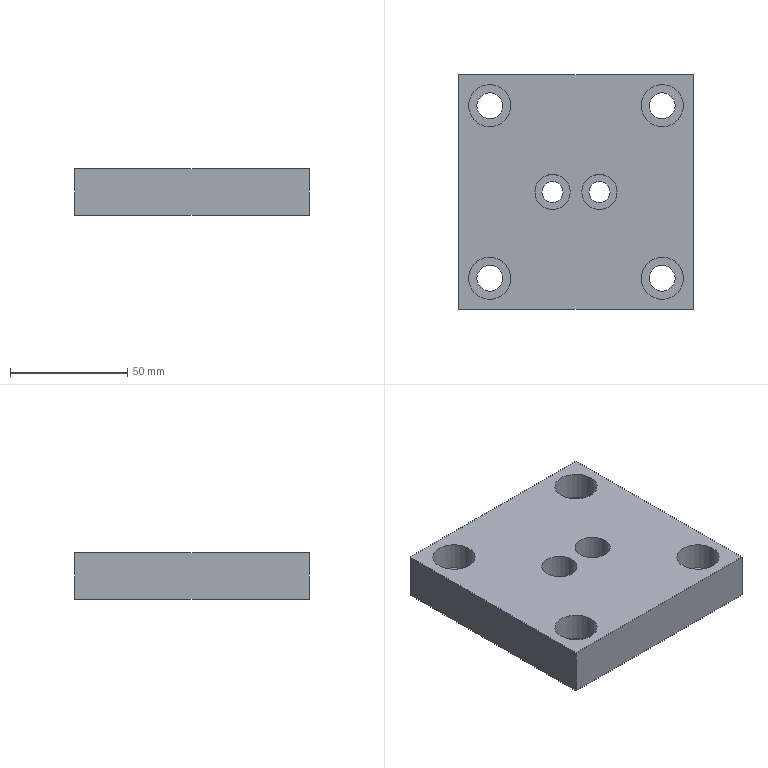Part | NX | features 1 2 | 1 solid | 24 faces | box 100 x 100 x 19.8 mm | volume 177134 mm3 | cylinder 12 | plane 12 | commonest cylinder face diameters 11 x4 18 x4 9 x2 15 x2
STEP:
#1=CARTESIAN_POINT('',(797.75,188.25,343.));
#2=VERTEX_POINT('',#1);
#3=CARTESIAN_POINT('',(806.75,188.25,343.));
#4=DIRECTION('',(0.,0.,-1.));
#5=DIRECTION('',(-1.,0.,0.));
#6=AXIS2_PLACEMENT_3D('',#3,#4,#5);
#7=CIRCLE('',#6,9.);
#8=EDGE_CURVE('',#2,#2,#7,.T.);
#9=ORIENTED_EDGE('',*,*,#8,.T.);
#10=EDGE_LOOP('',(#9));
#11=FACE_BOUND('',#10,.T.);
#12=CARTESIAN_POINT('',(797.75,188.25,355.));
#13=VERTEX_POINT('',#12);
#14=CARTESIAN_POINT('',(806.75,188.25,355.));
#15=DIRECTION('',(0.,0.,1.));
#16=DIRECTION('',(-1.,0.,0.));
#17=AXIS2_PLACEMENT_3D('',#14,#15,#16);
#18=CIRCLE('',#17,9.);
#19=EDGE_CURVE('',#13,#13,#18,.T.);
#20=ORIENTED_EDGE('',*,*,#19,.T.);
#21=EDGE_LOOP('',(#20));
#22=FACE_BOUND('',#21,.T.);
#23=CARTESIAN_POINT('',(806.75,188.25,355.));
#24=DIRECTION('',(0.,0.,1.));
#25=DIRECTION('',(0.,-1.,0.));
#26=AXIS2_PLACEMENT_3D('',#23,#24,#25);
#27=CYLINDRICAL_SURFACE('',#26,9.);
#28=ADVANCED_FACE('',(#11,#22),#27,.F.);
#29=CARTESIAN_POINT('',(801.25,188.25,335.2));
#30=VERTEX_POINT('',#29);
#31=CARTESIAN_POINT('',(806.75,188.25,335.2));
#32=DIRECTION('',(0.,0.,-1.));
#33=DIRECTION('',(-1.,0.,0.));
#34=AXIS2_PLACEMENT_3D('',#31,#32,#33);
#35=CIRCLE('',#34,5.5);
#36=EDGE_CURVE('',#30,#30,#35,.T.);
#37=ORIENTED_EDGE('',*,*,#36,.T.);
#38=EDGE_LOOP('',(#37));
#39=FACE_BOUND('',#38,.T.);
#40=CARTESIAN_POINT('',(801.25,188.25,343.));
#41=VERTEX_POINT('',#40);
#42=CARTESIAN_POINT('',(806.75,188.25,343.));
#43=DIRECTION('',(0.,0.,1.));
#44=DIRECTION('',(-1.,0.,0.));
#45=AXIS2_PLACEMENT_3D('',#42,#43,#44);
#46=CIRCLE('',#45,5.5);
#47=EDGE_CURVE('',#41,#41,#46,.T.);
#48=ORIENTED_EDGE('',*,*,#47,.T.);
#49=EDGE_LOOP('',(#48));
#50=FACE_BOUND('',#49,.T.);
#51=CARTESIAN_POINT('',(806.75,188.25,343.));
#52=DIRECTION('',(0.,0.,1.));
#53=DIRECTION('',(0.,-1.,0.));
#54=AXIS2_PLACEMENT_3D('',#51,#52,#53);
#55=CYLINDRICAL_SURFACE('',#54,5.5);
#56=ADVANCED_FACE('',(#39,#50),#55,.F.);
#57=CARTESIAN_POINT('',(724.25,188.25,343.));
#58=VERTEX_POINT('',#57);
#59=CARTESIAN_POINT('',(733.25,188.25,343.));
#60=DIRECTION('',(0.,0.,-1.));
#61=DIRECTION('',(-1.,0.,0.));
#62=AXIS2_PLACEMENT_3D('',#59,#60,#61);
#63=CIRCLE('',#62,9.);
#64=EDGE_CURVE('',#58,#58,#63,.T.);
#65=ORIENTED_EDGE('',*,*,#64,.T.);
#66=EDGE_LOOP('',(#65));
#67=FACE_BOUND('',#66,.T.);
#68=CARTESIAN_POINT('',(724.25,188.25,355.));
#69=VERTEX_POINT('',#68);
#70=CARTESIAN_POINT('',(733.25,188.25,355.));
#71=DIRECTION('',(0.,0.,1.));
#72=DIRECTION('',(-1.,0.,0.));
#73=AXIS2_PLACEMENT_3D('',#70,#71,#72);
#74=CIRCLE('',#73,9.);
#75=EDGE_CURVE('',#69,#69,#74,.T.);
#76=ORIENTED_EDGE('',*,*,#75,.T.);
#77=EDGE_LOOP('',(#76));
#78=FACE_BOUND('',#77,.T.);
#79=CARTESIAN_POINT('',(733.25,188.25,355.));
#80=DIRECTION('',(0.,0.,1.));
#81=DIRECTION('',(0.,-1.,0.));
#82=AXIS2_PLACEMENT_3D('',#79,#80,#81);
#83=CYLINDRICAL_SURFACE('',#82,9.);
#84=ADVANCED_FACE('',(#67,#78),#83,.F.);
#85=CARTESIAN_POINT('',(727.75,188.25,335.2));
#86=VERTEX_POINT('',#85);
#87=CARTESIAN_POINT('',(733.25,188.25,335.2));
#88=DIRECTION('',(0.,0.,-1.));
#89=DIRECTION('',(-1.,0.,0.));
#90=AXIS2_PLACEMENT_3D('',#87,#88,#89);
#91=CIRCLE('',#90,5.5);
#92=EDGE_CURVE('',#86,#86,#91,.T.);
#93=ORIENTED_EDGE('',*,*,#92,.T.);
#94=EDGE_LOOP('',(#93));
#95=FACE_BOUND('',#94,.T.);
#96=CARTESIAN_POINT('',(727.75,188.25,343.));
#97=VERTEX_POINT('',#96);
#98=CARTESIAN_POINT('',(733.25,188.25,343.));
#99=DIRECTION('',(0.,0.,1.));
#100=DIRECTION('',(-1.,0.,0.));
#101=AXIS2_PLACEMENT_3D('',#98,#99,#100);
#102=CIRCLE('',#101,5.5);
#103=EDGE_CURVE('',#97,#97,#102,.T.);
#104=ORIENTED_EDGE('',*,*,#103,.T.);
#105=EDGE_LOOP('',(#104));
#106=FACE_BOUND('',#105,.T.);
#107=CARTESIAN_POINT('',(733.25,188.25,343.));
#108=DIRECTION('',(0.,0.,1.));
#109=DIRECTION('',(0.,-1.,0.));
#110=AXIS2_PLACEMENT_3D('',#107,#108,#109);
#111=CYLINDRICAL_SURFACE('',#110,5.5);
#112=ADVANCED_FACE('',(#95,#106),#111,.F.);
#113=CARTESIAN_POINT('',(797.75,261.75,343.));
#114=VERTEX_POINT('',#113);
#115=CARTESIAN_POINT('',(806.75,261.75,343.));
#116=DIRECTION('',(0.,0.,-1.));
#117=DIRECTION('',(-1.,0.,0.));
#118=AXIS2_PLACEMENT_3D('',#115,#116,#117);
#119=CIRCLE('',#118,9.);
#120=EDGE_CURVE('',#114,#114,#119,.T.);
#121=ORIENTED_EDGE('',*,*,#120,.T.);
#122=EDGE_LOOP('',(#121));
#123=FACE_BOUND('',#122,.T.);
#124=CARTESIAN_POINT('',(797.75,261.75,355.));
#125=VERTEX_POINT('',#124);
#126=CARTESIAN_POINT('',(806.75,261.75,355.));
#127=DIRECTION('',(0.,0.,1.));
#128=DIRECTION('',(-1.,0.,0.));
#129=AXIS2_PLACEMENT_3D('',#126,#127,#128);
#130=CIRCLE('',#129,9.);
#131=EDGE_CURVE('',#125,#125,#130,.T.);
#132=ORIENTED_EDGE('',*,*,#131,.T.);
#133=EDGE_LOOP('',(#132));
#134=FACE_BOUND('',#133,.T.);
#135=CARTESIAN_POINT('',(806.75,261.75,355.));
#136=DIRECTION('',(0.,0.,1.));
#137=DIRECTION('',(0.,-1.,0.));
#138=AXIS2_PLACEMENT_3D('',#135,#136,#137);
#139=CYLINDRICAL_SURFACE('',#138,9.);
#140=ADVANCED_FACE('',(#123,#134),#139,.F.);
#141=CARTESIAN_POINT('',(801.25,261.75,335.2));
#142=VERTEX_POINT('',#141);
#143=CARTESIAN_POINT('',(806.75,261.75,335.2));
#144=DIRECTION('',(0.,0.,-1.));
#145=DIRECTION('',(-1.,0.,0.));
#146=AXIS2_PLACEMENT_3D('',#143,#144,#145);
#147=CIRCLE('',#146,5.5);
#148=EDGE_CURVE('',#142,#142,#147,.T.);
#149=ORIENTED_EDGE('',*,*,#148,.T.);
#150=EDGE_LOOP('',(#149));
#151=FACE_BOUND('',#150,.T.);
#152=CARTESIAN_POINT('',(801.25,261.75,343.));
#153=VERTEX_POINT('',#152);
#154=CARTESIAN_POINT('',(806.75,261.75,343.));
#155=DIRECTION('',(0.,0.,1.));
#156=DIRECTION('',(-1.,0.,0.));
#157=AXIS2_PLACEMENT_3D('',#154,#155,#156);
#158=CIRCLE('',#157,5.5);
#159=EDGE_CURVE('',#153,#153,#158,.T.);
#160=ORIENTED_EDGE('',*,*,#159,.T.);
#161=EDGE_LOOP('',(#160));
#162=FACE_BOUND('',#161,.T.);
#163=CARTESIAN_POINT('',(806.75,261.75,343.));
#164=DIRECTION('',(0.,0.,1.));
#165=DIRECTION('',(0.,-1.,0.));
#166=AXIS2_PLACEMENT_3D('',#163,#164,#165);
#167=CYLINDRICAL_SURFACE('',#166,5.5);
#168=ADVANCED_FACE('',(#151,#162),#167,.F.);
#169=CARTESIAN_POINT('',(724.25,261.75,343.));
#170=VERTEX_POINT('',#169);
#171=CARTESIAN_POINT('',(733.25,261.75,343.));
#172=DIRECTION('',(0.,0.,-1.));
#173=DIRECTION('',(-1.,0.,0.));
#174=AXIS2_PLACEMENT_3D('',#171,#172,#173);
#175=CIRCLE('',#174,9.);
#176=EDGE_CURVE('',#170,#170,#175,.T.);
#177=ORIENTED_EDGE('',*,*,#176,.T.);
#178=EDGE_LOOP('',(#177));
#179=FACE_BOUND('',#178,.T.);
#180=CARTESIAN_POINT('',(724.25,261.75,355.));
#181=VERTEX_POINT('',#180);
#182=CARTESIAN_POINT('',(733.25,261.75,355.));
#183=DIRECTION('',(0.,0.,1.));
#184=DIRECTION('',(-1.,0.,0.));
#185=AXIS2_PLACEMENT_3D('',#182,#183,#184);
#186=CIRCLE('',#185,9.);
#187=EDGE_CURVE('',#181,#181,#186,.T.);
#188=ORIENTED_EDGE('',*,*,#187,.T.);
#189=EDGE_LOOP('',(#188));
#190=FACE_BOUND('',#189,.T.);
#191=CARTESIAN_POINT('',(733.25,261.75,355.));
#192=DIRECTION('',(0.,0.,1.));
#193=DIRECTION('',(0.,-1.,0.));
#194=AXIS2_PLACEMENT_3D('',#191,#192,#193);
#195=CYLINDRICAL_SURFACE('',#194,9.);
#196=ADVANCED_FACE('',(#179,#190),#195,.F.);
#197=CARTESIAN_POINT('',(727.75,261.75,335.2));
#198=VERTEX_POINT('',#197);
#199=CARTESIAN_POINT('',(733.25,261.75,335.2));
#200=DIRECTION('',(0.,0.,-1.));
#201=DIRECTION('',(-1.,0.,0.));
#202=AXIS2_PLACEMENT_3D('',#199,#200,#201);
#203=CIRCLE('',#202,5.5);
#204=EDGE_CURVE('',#198,#198,#203,.T.);
#205=ORIENTED_EDGE('',*,*,#204,.T.);
#206=EDGE_LOOP('',(#205));
#207=FACE_BOUND('',#206,.T.);
#208=CARTESIAN_POINT('',(727.75,261.75,343.));
#209=VERTEX_POINT('',#208);
#210=CARTESIAN_POINT('',(733.25,261.75,343.));
#211=DIRECTION('',(0.,0.,1.));
#212=DIRECTION('',(-1.,0.,0.));
#213=AXIS2_PLACEMENT_3D('',#210,#211,#212);
#214=CIRCLE('',#213,5.5);
#215=EDGE_CURVE('',#209,#209,#214,.T.);
#216=ORIENTED_EDGE('',*,*,#215,.T.);
#217=EDGE_LOOP('',(#216));
#218=FACE_BOUND('',#217,.T.);
#219=CARTESIAN_POINT('',(733.25,261.75,343.));
#220=DIRECTION('',(0.,0.,1.));
#221=DIRECTION('',(0.,-1.,0.));
#222=AXIS2_PLACEMENT_3D('',#219,#220,#221);
#223=CYLINDRICAL_SURFACE('',#222,5.5);
#224=ADVANCED_FACE('',(#207,#218),#223,.F.);
#225=CARTESIAN_POINT('',(772.5,225.,341.));
#226=VERTEX_POINT('',#225);
#227=CARTESIAN_POINT('',(780.,225.,341.));
#228=DIRECTION('',(0.,0.,-1.));
#229=DIRECTION('',(-1.,0.,0.));
#230=AXIS2_PLACEMENT_3D('',#227,#228,#229);
#231=CIRCLE('',#230,7.5);
#232=EDGE_CURVE('',#226,#226,#231,.T.);
#233=ORIENTED_EDGE('',*,*,#232,.T.);
#234=EDGE_LOOP('',(#233));
#235=FACE_BOUND('',#234,.T.);
#236=CARTESIAN_POINT('',(772.5,225.,355.));
#237=VERTEX_POINT('',#236);
#238=CARTESIAN_POINT('',(780.,225.,355.));
#239=DIRECTION('',(0.,0.,1.));
#240=DIRECTION('',(-1.,0.,0.));
#241=AXIS2_PLACEMENT_3D('',#238,#239,#240);
#242=CIRCLE('',#241,7.5);
#243=EDGE_CURVE('',#237,#237,#242,.T.);
#244=ORIENTED_EDGE('',*,*,#243,.T.);
#245=EDGE_LOOP('',(#244));
#246=FACE_BOUND('',#245,.T.);
#247=CARTESIAN_POINT('',(780.,225.,355.));
#248=DIRECTION('',(0.,0.,1.));
#249=DIRECTION('',(0.,-1.,0.));
#250=AXIS2_PLACEMENT_3D('',#247,#248,#249);
#251=CYLINDRICAL_SURFACE('',#250,7.5);
#252=ADVANCED_FACE('',(#235,#246),#251,.F.);
#253=CARTESIAN_POINT('',(775.5,225.,335.2));
#254=VERTEX_POINT('',#253);
#255=CARTESIAN_POINT('',(780.,225.,335.2));
#256=DIRECTION('',(0.,0.,-1.));
#257=DIRECTION('',(-1.,0.,0.));
#258=AXIS2_PLACEMENT_3D('',#255,#256,#257);
#259=CIRCLE('',#258,4.5);
#260=EDGE_CURVE('',#254,#254,#259,.T.);
#261=ORIENTED_EDGE('',*,*,#260,.T.);
#262=EDGE_LOOP('',(#261));
#263=FACE_BOUND('',#262,.T.);
#264=CARTESIAN_POINT('',(775.5,225.,341.));
#265=VERTEX_POINT('',#264);
#266=CARTESIAN_POINT('',(780.,225.,341.));
#267=DIRECTION('',(0.,0.,1.));
#268=DIRECTION('',(-1.,0.,0.));
#269=AXIS2_PLACEMENT_3D('',#266,#267,#268);
#270=CIRCLE('',#269,4.5);
#271=EDGE_CURVE('',#265,#265,#270,.T.);
#272=ORIENTED_EDGE('',*,*,#271,.T.);
#273=EDGE_LOOP('',(#272));
#274=FACE_BOUND('',#273,.T.);
#275=CARTESIAN_POINT('',(780.,225.,341.));
#276=DIRECTION('',(0.,0.,1.));
#277=DIRECTION('',(0.,-1.,0.));
#278=AXIS2_PLACEMENT_3D('',#275,#276,#277);
#279=CYLINDRICAL_SURFACE('',#278,4.5);
#280=ADVANCED_FACE('',(#263,#274),#279,.F.);
#281=CARTESIAN_POINT('',(752.5,225.,341.));
#282=VERTEX_POINT('',#281);
#283=CARTESIAN_POINT('',(760.,225.,341.));
#284=DIRECTION('',(0.,0.,-1.));
#285=DIRECTION('',(-1.,0.,0.));
#286=AXIS2_PLACEMENT_3D('',#283,#284,#285);
#287=CIRCLE('',#286,7.5);
#288=EDGE_CURVE('',#282,#282,#287,.T.);
#289=ORIENTED_EDGE('',*,*,#288,.T.);
#290=EDGE_LOOP('',(#289));
#291=FACE_BOUND('',#290,.T.);
#292=CARTESIAN_POINT('',(752.5,225.,355.));
#293=VERTEX_POINT('',#292);
#294=CARTESIAN_POINT('',(760.,225.,355.));
#295=DIRECTION('',(0.,0.,1.));
#296=DIRECTION('',(-1.,0.,0.));
#297=AXIS2_PLACEMENT_3D('',#294,#295,#296);
#298=CIRCLE('',#297,7.5);
#299=EDGE_CURVE('',#293,#293,#298,.T.);
#300=ORIENTED_EDGE('',*,*,#299,.T.);
#301=EDGE_LOOP('',(#300));
#302=FACE_BOUND('',#301,.T.);
#303=CARTESIAN_POINT('',(760.,225.,355.));
#304=DIRECTION('',(0.,0.,1.));
#305=DIRECTION('',(0.,-1.,0.));
#306=AXIS2_PLACEMENT_3D('',#303,#304,#305);
#307=CYLINDRICAL_SURFACE('',#306,7.5);
#308=ADVANCED_FACE('',(#291,#302),#307,.F.);
#309=CARTESIAN_POINT('',(755.5,225.,335.2));
#310=VERTEX_POINT('',#309);
#311=CARTESIAN_POINT('',(760.,225.,335.2));
#312=DIRECTION('',(0.,0.,-1.));
#313=DIRECTION('',(-1.,0.,0.));
#314=AXIS2_PLACEMENT_3D('',#311,#312,#313);
#315=CIRCLE('',#314,4.5);
#316=EDGE_CURVE('',#310,#310,#315,.T.);
#317=ORIENTED_EDGE('',*,*,#316,.T.);
#318=EDGE_LOOP('',(#317));
#319=FACE_BOUND('',#318,.T.);
#320=CARTESIAN_POINT('',(755.5,225.,341.));
#321=VERTEX_POINT('',#320);
#322=CARTESIAN_POINT('',(760.,225.,341.));
#323=DIRECTION('',(0.,0.,1.));
#324=DIRECTION('',(-1.,0.,0.));
#325=AXIS2_PLACEMENT_3D('',#322,#323,#324);
#326=CIRCLE('',#325,4.5);
#327=EDGE_CURVE('',#321,#321,#326,.T.);
#328=ORIENTED_EDGE('',*,*,#327,.T.);
#329=EDGE_LOOP('',(#328));
#330=FACE_BOUND('',#329,.T.);
#331=CARTESIAN_POINT('',(760.,225.,341.));
#332=DIRECTION('',(0.,0.,1.));
#333=DIRECTION('',(0.,-1.,0.));
#334=AXIS2_PLACEMENT_3D('',#331,#332,#333);
#335=CYLINDRICAL_SURFACE('',#334,4.5);
#336=ADVANCED_FACE('',(#319,#330),#335,.F.);
#337=ORIENTED_EDGE('',*,*,#327,.F.);
#338=EDGE_LOOP('',(#337));
#339=FACE_BOUND('',#338,.T.);
#340=ORIENTED_EDGE('',*,*,#288,.F.);
#341=EDGE_LOOP('',(#340));
#342=FACE_BOUND('',#341,.T.);
#343=CARTESIAN_POINT('',(820.,175.,341.));
#344=DIRECTION('',(0.,0.,1.));
#345=DIRECTION('',(0.,-1.,0.));
#346=AXIS2_PLACEMENT_3D('',#343,#344,#345);
#347=PLANE('',#346);
#348=ADVANCED_FACE('',(#339,#342),#347,.T.);
#349=ORIENTED_EDGE('',*,*,#271,.F.);
#350=EDGE_LOOP('',(#349));
#351=FACE_BOUND('',#350,.T.);
#352=ORIENTED_EDGE('',*,*,#232,.F.);
#353=EDGE_LOOP('',(#352));
#354=FACE_BOUND('',#353,.T.);
#355=CARTESIAN_POINT('',(820.,175.,341.));
#356=DIRECTION('',(0.,0.,1.));
#357=DIRECTION('',(0.,-1.,0.));
#358=AXIS2_PLACEMENT_3D('',#355,#356,#357);
#359=PLANE('',#358);
#360=ADVANCED_FACE('',(#351,#354),#359,.T.);
#361=ORIENTED_EDGE('',*,*,#215,.F.);
#362=EDGE_LOOP('',(#361));
#363=FACE_BOUND('',#362,.T.);
#364=ORIENTED_EDGE('',*,*,#176,.F.);
#365=EDGE_LOOP('',(#364));
#366=FACE_BOUND('',#365,.T.);
#367=CARTESIAN_POINT('',(820.,175.,343.));
#368=DIRECTION('',(0.,0.,1.));
#369=DIRECTION('',(0.,-1.,0.));
#370=AXIS2_PLACEMENT_3D('',#367,#368,#369);
#371=PLANE('',#370);
#372=ADVANCED_FACE('',(#363,#366),#371,.T.);
#373=ORIENTED_EDGE('',*,*,#159,.F.);
#374=EDGE_LOOP('',(#373));
#375=FACE_BOUND('',#374,.T.);
#376=ORIENTED_EDGE('',*,*,#120,.F.);
#377=EDGE_LOOP('',(#376));
#378=FACE_BOUND('',#377,.T.);
#379=CARTESIAN_POINT('',(820.,175.,343.));
#380=DIRECTION('',(0.,0.,1.));
#381=DIRECTION('',(0.,-1.,0.));
#382=AXIS2_PLACEMENT_3D('',#379,#380,#381);
#383=PLANE('',#382);
#384=ADVANCED_FACE('',(#375,#378),#383,.T.);
#385=ORIENTED_EDGE('',*,*,#103,.F.);
#386=EDGE_LOOP('',(#385));
#387=FACE_BOUND('',#386,.T.);
#388=ORIENTED_EDGE('',*,*,#64,.F.);
#389=EDGE_LOOP('',(#388));
#390=FACE_BOUND('',#389,.T.);
#391=CARTESIAN_POINT('',(820.,175.,343.));
#392=DIRECTION('',(0.,0.,1.));
#393=DIRECTION('',(0.,-1.,0.));
#394=AXIS2_PLACEMENT_3D('',#391,#392,#393);
#395=PLANE('',#394);
#396=ADVANCED_FACE('',(#387,#390),#395,.T.);
#397=ORIENTED_EDGE('',*,*,#47,.F.);
#398=EDGE_LOOP('',(#397));
#399=FACE_BOUND('',#398,.T.);
#400=ORIENTED_EDGE('',*,*,#8,.F.);
#401=EDGE_LOOP('',(#400));
#402=FACE_BOUND('',#401,.T.);
#403=CARTESIAN_POINT('',(820.,175.,343.));
#404=DIRECTION('',(0.,0.,1.));
#405=DIRECTION('',(0.,-1.,0.));
#406=AXIS2_PLACEMENT_3D('',#403,#404,#405);
#407=PLANE('',#406);
#408=ADVANCED_FACE('',(#399,#402),#407,.T.);
#409=CARTESIAN_POINT('',(820.,175.,335.2));
#410=VERTEX_POINT('',#409);
#411=CARTESIAN_POINT('',(720.,175.,335.2));
#412=VERTEX_POINT('',#411);
#413=CARTESIAN_POINT('',(720.,175.,335.2));
#414=DIRECTION('',(-1.,0.,0.));
#415=VECTOR('',#414,1000.);
#416=LINE('',#413,#415);
#417=EDGE_CURVE('',#410,#412,#416,.T.);
#418=ORIENTED_EDGE('',*,*,#417,.F.);
#419=CARTESIAN_POINT('',(820.,175.,355.));
#420=VERTEX_POINT('',#419);
#421=CARTESIAN_POINT('',(820.,175.,355.));
#422=DIRECTION('',(0.,0.,-1.));
#423=VECTOR('',#422,1000.);
#424=LINE('',#421,#423);
#425=EDGE_CURVE('',#420,#410,#424,.T.);
#426=ORIENTED_EDGE('',*,*,#425,.F.);
#427=CARTESIAN_POINT('',(720.,175.,355.));
#428=VERTEX_POINT('',#427);
#429=CARTESIAN_POINT('',(720.,175.,355.));
#430=DIRECTION('',(1.,0.,0.));
#431=VECTOR('',#430,1000.);
#432=LINE('',#429,#431);
#433=EDGE_CURVE('',#428,#420,#432,.T.);
#434=ORIENTED_EDGE('',*,*,#433,.F.);
#435=CARTESIAN_POINT('',(720.,175.,355.));
#436=DIRECTION('',(0.,0.,-1.));
#437=VECTOR('',#436,1000.);
#438=LINE('',#435,#437);
#439=EDGE_CURVE('',#428,#412,#438,.T.);
#440=ORIENTED_EDGE('',*,*,#439,.T.);
#441=EDGE_LOOP('',(#418,#426,#434,#440));
#442=FACE_BOUND('',#441,.T.);
#443=CARTESIAN_POINT('',(820.,175.,355.));
#444=DIRECTION('',(0.,-1.,0.));
#445=DIRECTION('',(1.,0.,0.));
#446=AXIS2_PLACEMENT_3D('',#443,#444,#445);
#447=PLANE('',#446);
#448=ADVANCED_FACE('',(#442),#447,.T.);
#449=CARTESIAN_POINT('',(720.,275.,335.2));
#450=VERTEX_POINT('',#449);
#451=CARTESIAN_POINT('',(720.,275.,335.2));
#452=DIRECTION('',(0.,1.,0.));
#453=VECTOR('',#452,1000.);
#454=LINE('',#451,#453);
#455=EDGE_CURVE('',#412,#450,#454,.T.);
#456=ORIENTED_EDGE('',*,*,#455,.F.);
#457=ORIENTED_EDGE('',*,*,#439,.F.);
#458=CARTESIAN_POINT('',(720.,275.,355.));
#459=VERTEX_POINT('',#458);
#460=CARTESIAN_POINT('',(720.,275.,355.));
#461=DIRECTION('',(0.,-1.,0.));
#462=VECTOR('',#461,1000.);
#463=LINE('',#460,#462);
#464=EDGE_CURVE('',#459,#428,#463,.T.);
#465=ORIENTED_EDGE('',*,*,#464,.F.);
#466=CARTESIAN_POINT('',(720.,275.,355.));
#467=DIRECTION('',(0.,0.,-1.));
#468=VECTOR('',#467,1000.);
#469=LINE('',#466,#468);
#470=EDGE_CURVE('',#459,#450,#469,.T.);
#471=ORIENTED_EDGE('',*,*,#470,.T.);
#472=EDGE_LOOP('',(#456,#457,#465,#471));
#473=FACE_BOUND('',#472,.T.);
#474=CARTESIAN_POINT('',(720.,175.,355.));
#475=DIRECTION('',(-1.,0.,0.));
#476=DIRECTION('',(0.,-1.,0.));
#477=AXIS2_PLACEMENT_3D('',#474,#475,#476);
#478=PLANE('',#477);
#479=ADVANCED_FACE('',(#473),#478,.T.);
#480=CARTESIAN_POINT('',(820.,275.,335.2));
#481=VERTEX_POINT('',#480);
#482=CARTESIAN_POINT('',(820.,275.,335.2));
#483=DIRECTION('',(1.,0.,0.));
#484=VECTOR('',#483,1000.);
#485=LINE('',#482,#484);
#486=EDGE_CURVE('',#450,#481,#485,.T.);
#487=ORIENTED_EDGE('',*,*,#486,.F.);
#488=ORIENTED_EDGE('',*,*,#470,.F.);
#489=CARTESIAN_POINT('',(820.,275.,355.));
#490=VERTEX_POINT('',#489);
#491=CARTESIAN_POINT('',(820.,275.,355.));
#492=DIRECTION('',(-1.,0.,0.));
#493=VECTOR('',#492,1000.);
#494=LINE('',#491,#493);
#495=EDGE_CURVE('',#490,#459,#494,.T.);
#496=ORIENTED_EDGE('',*,*,#495,.F.);
#497=CARTESIAN_POINT('',(820.,275.,355.));
#498=DIRECTION('',(0.,0.,-1.));
#499=VECTOR('',#498,1000.);
#500=LINE('',#497,#499);
#501=EDGE_CURVE('',#490,#481,#500,.T.);
#502=ORIENTED_EDGE('',*,*,#501,.T.);
#503=EDGE_LOOP('',(#487,#488,#496,#502));
#504=FACE_BOUND('',#503,.T.);
#505=CARTESIAN_POINT('',(720.,275.,355.));
#506=DIRECTION('',(0.,1.,0.));
#507=DIRECTION('',(-1.,0.,0.));
#508=AXIS2_PLACEMENT_3D('',#505,#506,#507);
#509=PLANE('',#508);
#510=ADVANCED_FACE('',(#504),#509,.T.);
#511=CARTESIAN_POINT('',(820.,175.,335.2));
#512=DIRECTION('',(0.,-1.,0.));
#513=VECTOR('',#512,1000.);
#514=LINE('',#511,#513);
#515=EDGE_CURVE('',#481,#410,#514,.T.);
#516=ORIENTED_EDGE('',*,*,#515,.F.);
#517=ORIENTED_EDGE('',*,*,#501,.F.);
#518=CARTESIAN_POINT('',(820.,175.,355.));
#519=DIRECTION('',(0.,1.,0.));
#520=VECTOR('',#519,1000.);
#521=LINE('',#518,#520);
#522=EDGE_CURVE('',#420,#490,#521,.T.);
#523=ORIENTED_EDGE('',*,*,#522,.F.);
#524=ORIENTED_EDGE('',*,*,#425,.T.);
#525=EDGE_LOOP('',(#516,#517,#523,#524));
#526=FACE_BOUND('',#525,.T.);
#527=CARTESIAN_POINT('',(820.,275.,355.));
#528=DIRECTION('',(1.,0.,0.));
#529=DIRECTION('',(0.,1.,0.));
#530=AXIS2_PLACEMENT_3D('',#527,#528,#529);
#531=PLANE('',#530);
#532=ADVANCED_FACE('',(#526),#531,.T.);
#533=ORIENTED_EDGE('',*,*,#316,.F.);
#534=EDGE_LOOP('',(#533));
#535=FACE_BOUND('',#534,.T.);
#536=ORIENTED_EDGE('',*,*,#260,.F.);
#537=EDGE_LOOP('',(#536));
#538=FACE_BOUND('',#537,.T.);
#539=ORIENTED_EDGE('',*,*,#204,.F.);
#540=EDGE_LOOP('',(#539));
#541=FACE_BOUND('',#540,.T.);
#542=ORIENTED_EDGE('',*,*,#148,.F.);
#543=EDGE_LOOP('',(#542));
#544=FACE_BOUND('',#543,.T.);
#545=ORIENTED_EDGE('',*,*,#92,.F.);
#546=EDGE_LOOP('',(#545));
#547=FACE_BOUND('',#546,.T.);
#548=ORIENTED_EDGE('',*,*,#36,.F.);
#549=EDGE_LOOP('',(#548));
#550=FACE_BOUND('',#549,.T.);
#551=ORIENTED_EDGE('',*,*,#417,.T.);
#552=ORIENTED_EDGE('',*,*,#455,.T.);
#553=ORIENTED_EDGE('',*,*,#486,.T.);
#554=ORIENTED_EDGE('',*,*,#515,.T.);
#555=EDGE_LOOP('',(#551,#552,#553,#554));
#556=FACE_BOUND('',#555,.T.);
#557=CARTESIAN_POINT('',(820.,175.,335.2));
#558=DIRECTION('',(0.,0.,-1.));
#559=DIRECTION('',(0.,1.,0.));
#560=AXIS2_PLACEMENT_3D('',#557,#558,#559);
#561=PLANE('',#560);
#562=ADVANCED_FACE('',(#535,#538,#541,#544,#547,#550,#556),#561,.T.);
#563=ORIENTED_EDGE('',*,*,#299,.F.);
#564=EDGE_LOOP('',(#563));
#565=FACE_BOUND('',#564,.T.);
#566=ORIENTED_EDGE('',*,*,#243,.F.);
#567=EDGE_LOOP('',(#566));
#568=FACE_BOUND('',#567,.T.);
#569=ORIENTED_EDGE('',*,*,#187,.F.);
#570=EDGE_LOOP('',(#569));
#571=FACE_BOUND('',#570,.T.);
#572=ORIENTED_EDGE('',*,*,#131,.F.);
#573=EDGE_LOOP('',(#572));
#574=FACE_BOUND('',#573,.T.);
#575=ORIENTED_EDGE('',*,*,#75,.F.);
#576=EDGE_LOOP('',(#575));
#577=FACE_BOUND('',#576,.T.);
#578=ORIENTED_EDGE('',*,*,#19,.F.);
#579=EDGE_LOOP('',(#578));
#580=FACE_BOUND('',#579,.T.);
#581=ORIENTED_EDGE('',*,*,#522,.T.);
#582=ORIENTED_EDGE('',*,*,#495,.T.);
#583=ORIENTED_EDGE('',*,*,#464,.T.);
#584=ORIENTED_EDGE('',*,*,#433,.T.);
#585=EDGE_LOOP('',(#581,#582,#583,#584));
#586=FACE_BOUND('',#585,.T.);
#587=CARTESIAN_POINT('',(820.,175.,355.));
#588=DIRECTION('',(0.,0.,-1.));
#589=DIRECTION('',(0.,1.,0.));
#590=AXIS2_PLACEMENT_3D('',#587,#588,#589);
#591=PLANE('',#590);
#592=ADVANCED_FACE('',(#565,#568,#571,#574,#577,#580,#586),#591,.F.);
#593=CLOSED_SHELL('',(#28,#56,#84,#112,#140,#168,#196,#224,#252,#280,#308,#336,#348,#360,#372,#384,#396,#408,#448,#479,#510,#532,#562,#592));
#594=MANIFOLD_SOLID_BREP('',#593);
#595=(LENGTH_UNIT()NAMED_UNIT(*)SI_UNIT(.MILLI.,.METRE.));
#596=UNCERTAINTY_MEASURE_WITH_UNIT(LENGTH_MEASURE(0.00001),#595,'','');
#597=(NAMED_UNIT(*)PLANE_ANGLE_UNIT()SI_UNIT($,.RADIAN.));
#598=(NAMED_UNIT(*)SI_UNIT($,.STERADIAN.)SOLID_ANGLE_UNIT());
#599=(GEOMETRIC_REPRESENTATION_CONTEXT(3)GLOBAL_UNCERTAINTY_ASSIGNED_CONTEXT((#596))GLOBAL_UNIT_ASSIGNED_CONTEXT((#595,#597,#598))REPRESENTATION_CONTEXT('',''));
#600=ADVANCED_BREP_SHAPE_REPRESENTATION('',(#594),#599);